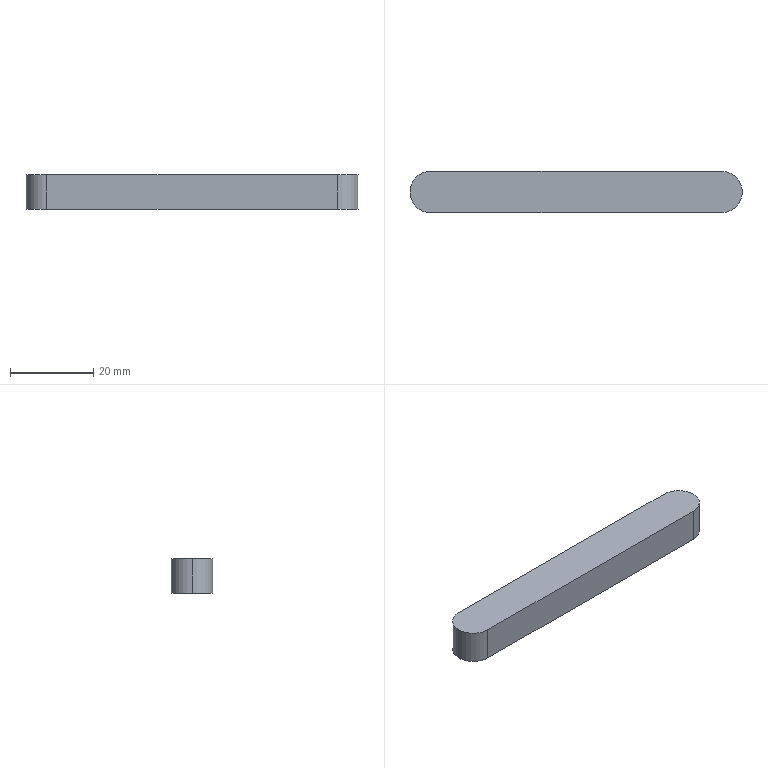Part | SolidWorks | features Extrusion 1 | 1 solid | 7 faces | box 80 x 10 x 8.3 mm | volume 6462 mm3 | plane 4 | cylinder 3 | commonest cylinder face diameters 10 x3
STEP:
#1=CARTESIAN_POINT('',(-5.,0.,8.3));
#2=VERTEX_POINT('',#1);
#3=CARTESIAN_POINT('',(0.,-5.,8.3));
#4=VERTEX_POINT('',#3);
#5=CARTESIAN_POINT('',(0.,0.,8.3));
#6=DIRECTION('',(0.,0.,1.));
#7=DIRECTION('',(1.,0.,0.));
#8=AXIS2_PLACEMENT_3D('',#5,#6,#7);
#9=CIRCLE('',#8,5.);
#10=EDGE_CURVE('',#2,#4,#9,.T.);
#11=ORIENTED_EDGE('',*,*,#10,.F.);
#12=CARTESIAN_POINT('',(-5.,0.,0.));
#13=VERTEX_POINT('',#12);
#14=CARTESIAN_POINT('',(-5.,0.,8.3));
#15=DIRECTION('',(0.,0.,-1.));
#16=VECTOR('',#15,1000.);
#17=LINE('',#14,#16);
#18=EDGE_CURVE('',#2,#13,#17,.T.);
#19=ORIENTED_EDGE('',*,*,#18,.T.);
#20=CARTESIAN_POINT('',(0.,-5.,0.));
#21=VERTEX_POINT('',#20);
#22=CARTESIAN_POINT('',(0.,0.,0.));
#23=DIRECTION('',(0.,0.,1.));
#24=DIRECTION('',(1.,0.,0.));
#25=AXIS2_PLACEMENT_3D('',#22,#23,#24);
#26=CIRCLE('',#25,5.);
#27=EDGE_CURVE('',#13,#21,#26,.T.);
#28=ORIENTED_EDGE('',*,*,#27,.T.);
#29=CARTESIAN_POINT('',(0.,-5.,8.3));
#30=DIRECTION('',(0.,0.,-1.));
#31=VECTOR('',#30,1000.);
#32=LINE('',#29,#31);
#33=EDGE_CURVE('',#4,#21,#32,.T.);
#34=ORIENTED_EDGE('',*,*,#33,.F.);
#35=EDGE_LOOP('',(#11,#19,#28,#34));
#36=FACE_OUTER_BOUND('',#35,.T.);
#37=CARTESIAN_POINT('',(0.,0.,8.3));
#38=DIRECTION('',(0.,0.,-1.));
#39=DIRECTION('',(-1.,0.,0.));
#40=AXIS2_PLACEMENT_3D('',#37,#38,#39);
#41=CYLINDRICAL_SURFACE('',#40,5.);
#42=ADVANCED_FACE('',(#36),#41,.T.);
#43=ORIENTED_EDGE('',*,*,#18,.F.);
#44=CARTESIAN_POINT('',(0.,5.,8.3));
#45=VERTEX_POINT('',#44);
#46=CARTESIAN_POINT('',(0.,0.,8.3));
#47=DIRECTION('',(0.,0.,1.));
#48=DIRECTION('',(1.,0.,0.));
#49=AXIS2_PLACEMENT_3D('',#46,#47,#48);
#50=CIRCLE('',#49,5.);
#51=EDGE_CURVE('',#45,#2,#50,.T.);
#52=ORIENTED_EDGE('',*,*,#51,.F.);
#53=CARTESIAN_POINT('',(0.,5.,0.));
#54=VERTEX_POINT('',#53);
#55=CARTESIAN_POINT('',(0.,5.,8.3));
#56=DIRECTION('',(0.,0.,-1.));
#57=VECTOR('',#56,1000.);
#58=LINE('',#55,#57);
#59=EDGE_CURVE('',#45,#54,#58,.T.);
#60=ORIENTED_EDGE('',*,*,#59,.T.);
#61=CARTESIAN_POINT('',(0.,0.,0.));
#62=DIRECTION('',(0.,0.,1.));
#63=DIRECTION('',(1.,0.,0.));
#64=AXIS2_PLACEMENT_3D('',#61,#62,#63);
#65=CIRCLE('',#64,5.);
#66=EDGE_CURVE('',#54,#13,#65,.T.);
#67=ORIENTED_EDGE('',*,*,#66,.T.);
#68=EDGE_LOOP('',(#43,#52,#60,#67));
#69=FACE_OUTER_BOUND('',#68,.T.);
#70=CARTESIAN_POINT('',(0.,0.,8.3));
#71=DIRECTION('',(0.,0.,-1.));
#72=DIRECTION('',(-1.,0.,0.));
#73=AXIS2_PLACEMENT_3D('',#70,#71,#72);
#74=CYLINDRICAL_SURFACE('',#73,5.);
#75=ADVANCED_FACE('',(#69),#74,.T.);
#76=CARTESIAN_POINT('',(70.,-5.,0.));
#77=VERTEX_POINT('',#76);
#78=CARTESIAN_POINT('',(0.,-5.,0.));
#79=DIRECTION('',(1.,0.,0.));
#80=VECTOR('',#79,1000.);
#81=LINE('',#78,#80);
#82=EDGE_CURVE('',#21,#77,#81,.T.);
#83=ORIENTED_EDGE('',*,*,#82,.T.);
#84=CARTESIAN_POINT('',(70.,-5.,8.3));
#85=VERTEX_POINT('',#84);
#86=CARTESIAN_POINT('',(70.,-5.,8.3));
#87=DIRECTION('',(0.,0.,-1.));
#88=VECTOR('',#87,1000.);
#89=LINE('',#86,#88);
#90=EDGE_CURVE('',#85,#77,#89,.T.);
#91=ORIENTED_EDGE('',*,*,#90,.F.);
#92=CARTESIAN_POINT('',(0.,-5.,8.3));
#93=DIRECTION('',(1.,0.,0.));
#94=VECTOR('',#93,1000.);
#95=LINE('',#92,#94);
#96=EDGE_CURVE('',#4,#85,#95,.T.);
#97=ORIENTED_EDGE('',*,*,#96,.F.);
#98=ORIENTED_EDGE('',*,*,#33,.T.);
#99=EDGE_LOOP('',(#83,#91,#97,#98));
#100=FACE_OUTER_BOUND('',#99,.T.);
#101=CARTESIAN_POINT('',(0.,-5.,8.3));
#102=DIRECTION('',(0.,1.,0.));
#103=DIRECTION('',(0.,0.,1.));
#104=AXIS2_PLACEMENT_3D('',#101,#102,#103);
#105=PLANE('',#104);
#106=ADVANCED_FACE('',(#100),#105,.F.);
#107=CARTESIAN_POINT('',(70.,5.,0.));
#108=VERTEX_POINT('',#107);
#109=CARTESIAN_POINT('',(70.,0.,0.));
#110=DIRECTION('',(0.,0.,1.));
#111=DIRECTION('',(1.,0.,0.));
#112=AXIS2_PLACEMENT_3D('',#109,#110,#111);
#113=CIRCLE('',#112,5.);
#114=EDGE_CURVE('',#77,#108,#113,.T.);
#115=ORIENTED_EDGE('',*,*,#114,.T.);
#116=CARTESIAN_POINT('',(70.,5.,8.3));
#117=VERTEX_POINT('',#116);
#118=CARTESIAN_POINT('',(70.,5.,8.3));
#119=DIRECTION('',(0.,0.,-1.));
#120=VECTOR('',#119,1000.);
#121=LINE('',#118,#120);
#122=EDGE_CURVE('',#117,#108,#121,.T.);
#123=ORIENTED_EDGE('',*,*,#122,.F.);
#124=CARTESIAN_POINT('',(70.,0.,8.3));
#125=DIRECTION('',(0.,0.,1.));
#126=DIRECTION('',(1.,0.,0.));
#127=AXIS2_PLACEMENT_3D('',#124,#125,#126);
#128=CIRCLE('',#127,5.);
#129=EDGE_CURVE('',#85,#117,#128,.T.);
#130=ORIENTED_EDGE('',*,*,#129,.F.);
#131=ORIENTED_EDGE('',*,*,#90,.T.);
#132=EDGE_LOOP('',(#115,#123,#130,#131));
#133=FACE_OUTER_BOUND('',#132,.T.);
#134=CARTESIAN_POINT('',(70.,0.,8.3));
#135=DIRECTION('',(0.,0.,-1.));
#136=DIRECTION('',(-1.,0.,0.));
#137=AXIS2_PLACEMENT_3D('',#134,#135,#136);
#138=CYLINDRICAL_SURFACE('',#137,5.);
#139=ADVANCED_FACE('',(#133),#138,.T.);
#140=CARTESIAN_POINT('',(0.,5.,0.));
#141=DIRECTION('',(-1.,0.,0.));
#142=VECTOR('',#141,1000.);
#143=LINE('',#140,#142);
#144=EDGE_CURVE('',#108,#54,#143,.T.);
#145=ORIENTED_EDGE('',*,*,#144,.T.);
#146=ORIENTED_EDGE('',*,*,#59,.F.);
#147=CARTESIAN_POINT('',(0.,5.,8.3));
#148=DIRECTION('',(-1.,0.,0.));
#149=VECTOR('',#148,1000.);
#150=LINE('',#147,#149);
#151=EDGE_CURVE('',#117,#45,#150,.T.);
#152=ORIENTED_EDGE('',*,*,#151,.F.);
#153=ORIENTED_EDGE('',*,*,#122,.T.);
#154=EDGE_LOOP('',(#145,#146,#152,#153));
#155=FACE_OUTER_BOUND('',#154,.T.);
#156=CARTESIAN_POINT('',(0.,5.,8.3));
#157=DIRECTION('',(0.,-1.,0.));
#158=DIRECTION('',(0.,0.,-1.));
#159=AXIS2_PLACEMENT_3D('',#156,#157,#158);
#160=PLANE('',#159);
#161=ADVANCED_FACE('',(#155),#160,.F.);
#162=ORIENTED_EDGE('',*,*,#51,.T.);
#163=ORIENTED_EDGE('',*,*,#10,.T.);
#164=ORIENTED_EDGE('',*,*,#96,.T.);
#165=ORIENTED_EDGE('',*,*,#129,.T.);
#166=ORIENTED_EDGE('',*,*,#151,.T.);
#167=EDGE_LOOP('',(#162,#163,#164,#165,#166));
#168=FACE_OUTER_BOUND('',#167,.T.);
#169=CARTESIAN_POINT('',(0.,0.,8.3));
#170=DIRECTION('',(0.,0.,1.));
#171=DIRECTION('',(1.,0.,0.));
#172=AXIS2_PLACEMENT_3D('',#169,#170,#171);
#173=PLANE('',#172);
#174=ADVANCED_FACE('',(#168),#173,.T.);
#175=ORIENTED_EDGE('',*,*,#66,.F.);
#176=ORIENTED_EDGE('',*,*,#144,.F.);
#177=ORIENTED_EDGE('',*,*,#114,.F.);
#178=ORIENTED_EDGE('',*,*,#82,.F.);
#179=ORIENTED_EDGE('',*,*,#27,.F.);
#180=EDGE_LOOP('',(#175,#176,#177,#178,#179));
#181=FACE_OUTER_BOUND('',#180,.T.);
#182=CARTESIAN_POINT('',(0.,0.,0.));
#183=DIRECTION('',(0.,0.,1.));
#184=DIRECTION('',(1.,0.,0.));
#185=AXIS2_PLACEMENT_3D('',#182,#183,#184);
#186=PLANE('',#185);
#187=ADVANCED_FACE('',(#181),#186,.F.);
#188=CLOSED_SHELL('',(#42,#75,#106,#139,#161,#174,#187));
#189=MANIFOLD_SOLID_BREP('',#188);
#190=CARTESIAN_POINT('',(0.,0.,0.));
#191=DIRECTION('',(0.,0.,1.));
#192=DIRECTION('',(1.,0.,0.));
#193=AXIS2_PLACEMENT_3D('',#190,#191,#192);
#194=(LENGTH_UNIT()NAMED_UNIT(*)SI_UNIT(.MILLI.,.METRE.));
#195=UNCERTAINTY_MEASURE_WITH_UNIT(LENGTH_MEASURE(0.00001),#194,'','');
#196=(NAMED_UNIT(*)PLANE_ANGLE_UNIT()SI_UNIT($,.RADIAN.));
#197=(NAMED_UNIT(*)SI_UNIT($,.STERADIAN.)SOLID_ANGLE_UNIT());
#198=(GEOMETRIC_REPRESENTATION_CONTEXT(3)GLOBAL_UNCERTAINTY_ASSIGNED_CONTEXT((#195))GLOBAL_UNIT_ASSIGNED_CONTEXT((#194,#196,#197))REPRESENTATION_CONTEXT('',''));
#199=ADVANCED_BREP_SHAPE_REPRESENTATION('',(#189,#193),#198);